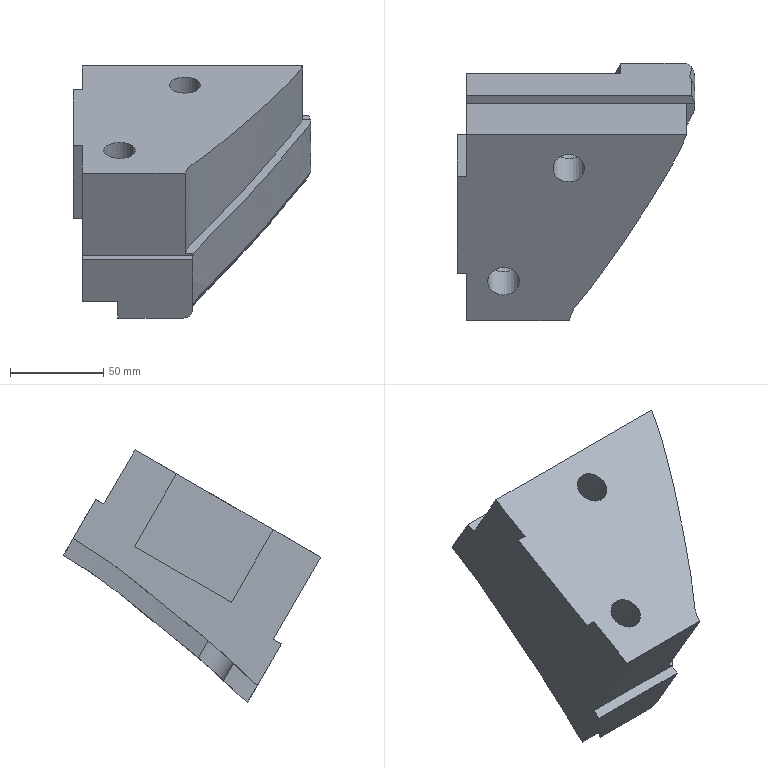Part | NX | features solid 2 | 1 solid | 31 faces | box 127.662 x 138.497 x 135.305 mm | volume 710077 mm3 | spline 14 | plane 13 | cylinder 4 | commonest cylinder face diameters 17 x2 25 x2